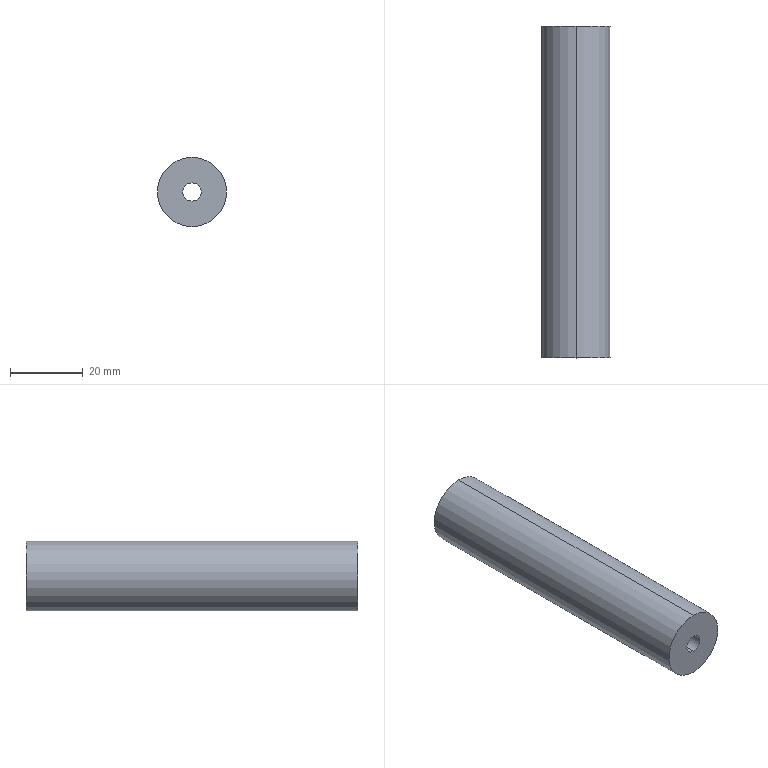Part | SolidWorks | features Extrusion 1, HoleWzd 1, ICE 1 | 1 solid | 9 faces | box 19 x 91 x 19 mm | volume 18359 mm3 | cylinder 6 | plane 3 | commonest cylinder face diameters 5 x2 11 x2 19 x2
STEP:
#1=CARTESIAN_POINT('',(0.,16.,-2.5));
#2=VERTEX_POINT('',#1);
#3=CARTESIAN_POINT('',(0.,16.,2.5));
#4=VERTEX_POINT('',#3);
#5=CARTESIAN_POINT('',(0.,16.,0.));
#6=DIRECTION('',(0.,1.,0.));
#7=DIRECTION('',(0.,0.,1.));
#8=AXIS2_PLACEMENT_3D('',#5,#6,#7);
#9=CIRCLE('',#8,2.5);
#10=EDGE_CURVE('',#2,#4,#9,.T.);
#11=ORIENTED_EDGE('',*,*,#10,.T.);
#12=CARTESIAN_POINT('',(0.,0.,2.5));
#13=VERTEX_POINT('',#12);
#14=CARTESIAN_POINT('',(0.,0.,2.5));
#15=DIRECTION('',(0.,-1.,0.));
#16=VECTOR('',#15,1000.);
#17=LINE('',#14,#16);
#18=EDGE_CURVE('',#4,#13,#17,.T.);
#19=ORIENTED_EDGE('',*,*,#18,.T.);
#20=CARTESIAN_POINT('',(0.,0.,-2.5));
#21=VERTEX_POINT('',#20);
#22=CARTESIAN_POINT('',(0.,0.,0.));
#23=DIRECTION('',(0.,-1.,0.));
#24=DIRECTION('',(0.,0.,-1.));
#25=AXIS2_PLACEMENT_3D('',#22,#23,#24);
#26=CIRCLE('',#25,2.5);
#27=EDGE_CURVE('',#13,#21,#26,.T.);
#28=ORIENTED_EDGE('',*,*,#27,.T.);
#29=CARTESIAN_POINT('',(0.,0.,-2.5));
#30=DIRECTION('',(0.,-1.,0.));
#31=VECTOR('',#30,1000.);
#32=LINE('',#29,#31);
#33=EDGE_CURVE('',#2,#21,#32,.T.);
#34=ORIENTED_EDGE('',*,*,#33,.F.);
#35=EDGE_LOOP('',(#11,#19,#28,#34));
#36=FACE_OUTER_BOUND('',#35,.T.);
#37=CARTESIAN_POINT('',(0.,0.,0.));
#38=DIRECTION('',(0.,-1.,0.));
#39=DIRECTION('',(0.,0.,-1.));
#40=AXIS2_PLACEMENT_3D('',#37,#38,#39);
#41=CYLINDRICAL_SURFACE('',#40,2.5);
#42=ADVANCED_FACE('',(#36),#41,.F.);
#43=CARTESIAN_POINT('',(0.,16.,-5.5));
#44=VERTEX_POINT('',#43);
#45=CARTESIAN_POINT('',(0.,16.,5.5));
#46=VERTEX_POINT('',#45);
#47=CARTESIAN_POINT('',(0.,16.,0.));
#48=DIRECTION('',(0.,1.,0.));
#49=DIRECTION('',(0.,0.,1.));
#50=AXIS2_PLACEMENT_3D('',#47,#48,#49);
#51=CIRCLE('',#50,5.5);
#52=EDGE_CURVE('',#44,#46,#51,.T.);
#53=ORIENTED_EDGE('',*,*,#52,.F.);
#54=CARTESIAN_POINT('',(0.,91.,-5.5));
#55=VERTEX_POINT('',#54);
#56=CARTESIAN_POINT('',(0.,16.,-5.5));
#57=DIRECTION('',(0.,1.,0.));
#58=VECTOR('',#57,1000.);
#59=LINE('',#56,#58);
#60=EDGE_CURVE('',#44,#55,#59,.T.);
#61=ORIENTED_EDGE('',*,*,#60,.T.);
#62=CARTESIAN_POINT('',(0.,91.,5.5));
#63=VERTEX_POINT('',#62);
#64=CARTESIAN_POINT('',(0.,91.,0.));
#65=DIRECTION('',(0.,1.,0.));
#66=DIRECTION('',(0.,0.,1.));
#67=AXIS2_PLACEMENT_3D('',#64,#65,#66);
#68=CIRCLE('',#67,5.5);
#69=EDGE_CURVE('',#55,#63,#68,.T.);
#70=ORIENTED_EDGE('',*,*,#69,.T.);
#71=CARTESIAN_POINT('',(0.,16.,5.5));
#72=DIRECTION('',(0.,1.,0.));
#73=VECTOR('',#72,1000.);
#74=LINE('',#71,#73);
#75=EDGE_CURVE('',#46,#63,#74,.T.);
#76=ORIENTED_EDGE('',*,*,#75,.F.);
#77=EDGE_LOOP('',(#53,#61,#70,#76));
#78=FACE_OUTER_BOUND('',#77,.T.);
#79=CARTESIAN_POINT('',(0.,16.,0.));
#80=DIRECTION('',(0.,1.,0.));
#81=DIRECTION('',(0.,0.,1.));
#82=AXIS2_PLACEMENT_3D('',#79,#80,#81);
#83=CYLINDRICAL_SURFACE('',#82,5.5);
#84=ADVANCED_FACE('',(#78),#83,.F.);
#85=CARTESIAN_POINT('',(0.,91.,9.5));
#86=VERTEX_POINT('',#85);
#87=CARTESIAN_POINT('',(0.,91.,-9.5));
#88=VERTEX_POINT('',#87);
#89=CARTESIAN_POINT('',(0.,91.,0.));
#90=DIRECTION('',(0.,1.,0.));
#91=DIRECTION('',(0.,0.,1.));
#92=AXIS2_PLACEMENT_3D('',#89,#90,#91);
#93=CIRCLE('',#92,9.5);
#94=EDGE_CURVE('',#86,#88,#93,.T.);
#95=ORIENTED_EDGE('',*,*,#94,.F.);
#96=CARTESIAN_POINT('',(0.,0.,9.5));
#97=VERTEX_POINT('',#96);
#98=CARTESIAN_POINT('',(0.,91.,9.5));
#99=DIRECTION('',(0.,-1.,0.));
#100=VECTOR('',#99,1000.);
#101=LINE('',#98,#100);
#102=EDGE_CURVE('',#86,#97,#101,.T.);
#103=ORIENTED_EDGE('',*,*,#102,.T.);
#104=CARTESIAN_POINT('',(0.,0.,-9.5));
#105=VERTEX_POINT('',#104);
#106=CARTESIAN_POINT('',(0.,0.,0.));
#107=DIRECTION('',(0.,1.,0.));
#108=DIRECTION('',(0.,0.,1.));
#109=AXIS2_PLACEMENT_3D('',#106,#107,#108);
#110=CIRCLE('',#109,9.5);
#111=EDGE_CURVE('',#97,#105,#110,.T.);
#112=ORIENTED_EDGE('',*,*,#111,.T.);
#113=CARTESIAN_POINT('',(0.,91.,-9.5));
#114=DIRECTION('',(0.,-1.,0.));
#115=VECTOR('',#114,1000.);
#116=LINE('',#113,#115);
#117=EDGE_CURVE('',#88,#105,#116,.T.);
#118=ORIENTED_EDGE('',*,*,#117,.F.);
#119=EDGE_LOOP('',(#95,#103,#112,#118));
#120=FACE_OUTER_BOUND('',#119,.T.);
#121=CARTESIAN_POINT('',(0.,91.,0.));
#122=DIRECTION('',(0.,-1.,0.));
#123=DIRECTION('',(0.,0.,-1.));
#124=AXIS2_PLACEMENT_3D('',#121,#122,#123);
#125=CYLINDRICAL_SURFACE('',#124,9.5);
#126=ADVANCED_FACE('',(#120),#125,.T.);
#127=ORIENTED_EDGE('',*,*,#102,.F.);
#128=CARTESIAN_POINT('',(0.,91.,0.));
#129=DIRECTION('',(0.,1.,0.));
#130=DIRECTION('',(0.,0.,1.));
#131=AXIS2_PLACEMENT_3D('',#128,#129,#130);
#132=CIRCLE('',#131,9.5);
#133=EDGE_CURVE('',#88,#86,#132,.T.);
#134=ORIENTED_EDGE('',*,*,#133,.F.);
#135=ORIENTED_EDGE('',*,*,#117,.T.);
#136=CARTESIAN_POINT('',(0.,0.,0.));
#137=DIRECTION('',(0.,1.,0.));
#138=DIRECTION('',(0.,0.,1.));
#139=AXIS2_PLACEMENT_3D('',#136,#137,#138);
#140=CIRCLE('',#139,9.5);
#141=EDGE_CURVE('',#105,#97,#140,.T.);
#142=ORIENTED_EDGE('',*,*,#141,.T.);
#143=EDGE_LOOP('',(#127,#134,#135,#142));
#144=FACE_OUTER_BOUND('',#143,.T.);
#145=CARTESIAN_POINT('',(0.,91.,0.));
#146=DIRECTION('',(0.,-1.,0.));
#147=DIRECTION('',(0.,0.,-1.));
#148=AXIS2_PLACEMENT_3D('',#145,#146,#147);
#149=CYLINDRICAL_SURFACE('',#148,9.5);
#150=ADVANCED_FACE('',(#144),#149,.T.);
#151=CARTESIAN_POINT('',(0.,91.,0.));
#152=DIRECTION('',(0.,1.,0.));
#153=DIRECTION('',(0.,0.,1.));
#154=AXIS2_PLACEMENT_3D('',#151,#152,#153);
#155=CIRCLE('',#154,5.5);
#156=EDGE_CURVE('',#63,#55,#155,.T.);
#157=ORIENTED_EDGE('',*,*,#156,.F.);
#158=ORIENTED_EDGE('',*,*,#69,.F.);
#159=EDGE_LOOP('',(#157,#158));
#160=FACE_BOUND('',#159,.T.);
#161=ORIENTED_EDGE('',*,*,#133,.T.);
#162=ORIENTED_EDGE('',*,*,#94,.T.);
#163=EDGE_LOOP('',(#161,#162));
#164=FACE_OUTER_BOUND('',#163,.T.);
#165=CARTESIAN_POINT('',(0.,91.,0.));
#166=DIRECTION('',(0.,1.,0.));
#167=DIRECTION('',(0.,0.,1.));
#168=AXIS2_PLACEMENT_3D('',#165,#166,#167);
#169=PLANE('',#168);
#170=ADVANCED_FACE('',(#160,#164),#169,.T.);
#171=CARTESIAN_POINT('',(0.,0.,0.));
#172=DIRECTION('',(0.,-1.,0.));
#173=DIRECTION('',(0.,0.,-1.));
#174=AXIS2_PLACEMENT_3D('',#171,#172,#173);
#175=CIRCLE('',#174,2.5);
#176=EDGE_CURVE('',#21,#13,#175,.T.);
#177=ORIENTED_EDGE('',*,*,#176,.F.);
#178=ORIENTED_EDGE('',*,*,#27,.F.);
#179=EDGE_LOOP('',(#177,#178));
#180=FACE_BOUND('',#179,.T.);
#181=ORIENTED_EDGE('',*,*,#141,.F.);
#182=ORIENTED_EDGE('',*,*,#111,.F.);
#183=EDGE_LOOP('',(#181,#182));
#184=FACE_OUTER_BOUND('',#183,.T.);
#185=CARTESIAN_POINT('',(0.,0.,0.));
#186=DIRECTION('',(0.,1.,0.));
#187=DIRECTION('',(0.,0.,1.));
#188=AXIS2_PLACEMENT_3D('',#185,#186,#187);
#189=PLANE('',#188);
#190=ADVANCED_FACE('',(#180,#184),#189,.F.);
#191=ORIENTED_EDGE('',*,*,#60,.F.);
#192=CARTESIAN_POINT('',(0.,16.,0.));
#193=DIRECTION('',(0.,1.,0.));
#194=DIRECTION('',(0.,0.,1.));
#195=AXIS2_PLACEMENT_3D('',#192,#193,#194);
#196=CIRCLE('',#195,5.5);
#197=EDGE_CURVE('',#46,#44,#196,.T.);
#198=ORIENTED_EDGE('',*,*,#197,.F.);
#199=ORIENTED_EDGE('',*,*,#75,.T.);
#200=ORIENTED_EDGE('',*,*,#156,.T.);
#201=EDGE_LOOP('',(#191,#198,#199,#200));
#202=FACE_OUTER_BOUND('',#201,.T.);
#203=CARTESIAN_POINT('',(0.,16.,0.));
#204=DIRECTION('',(0.,1.,0.));
#205=DIRECTION('',(0.,0.,1.));
#206=AXIS2_PLACEMENT_3D('',#203,#204,#205);
#207=CYLINDRICAL_SURFACE('',#206,5.5);
#208=ADVANCED_FACE('',(#202),#207,.F.);
#209=ORIENTED_EDGE('',*,*,#10,.F.);
#210=CARTESIAN_POINT('',(0.,16.,0.));
#211=DIRECTION('',(0.,1.,0.));
#212=DIRECTION('',(0.,0.,1.));
#213=AXIS2_PLACEMENT_3D('',#210,#211,#212);
#214=CIRCLE('',#213,2.5);
#215=EDGE_CURVE('',#4,#2,#214,.T.);
#216=ORIENTED_EDGE('',*,*,#215,.F.);
#217=EDGE_LOOP('',(#209,#216));
#218=FACE_BOUND('',#217,.T.);
#219=ORIENTED_EDGE('',*,*,#197,.T.);
#220=ORIENTED_EDGE('',*,*,#52,.T.);
#221=EDGE_LOOP('',(#219,#220));
#222=FACE_OUTER_BOUND('',#221,.T.);
#223=CARTESIAN_POINT('',(0.,16.,0.));
#224=DIRECTION('',(0.,1.,0.));
#225=DIRECTION('',(0.,0.,1.));
#226=AXIS2_PLACEMENT_3D('',#223,#224,#225);
#227=PLANE('',#226);
#228=ADVANCED_FACE('',(#218,#222),#227,.T.);
#229=ORIENTED_EDGE('',*,*,#18,.F.);
#230=ORIENTED_EDGE('',*,*,#215,.T.);
#231=ORIENTED_EDGE('',*,*,#33,.T.);
#232=ORIENTED_EDGE('',*,*,#176,.T.);
#233=EDGE_LOOP('',(#229,#230,#231,#232));
#234=FACE_OUTER_BOUND('',#233,.T.);
#235=CARTESIAN_POINT('',(0.,0.,0.));
#236=DIRECTION('',(0.,-1.,0.));
#237=DIRECTION('',(0.,0.,-1.));
#238=AXIS2_PLACEMENT_3D('',#235,#236,#237);
#239=CYLINDRICAL_SURFACE('',#238,2.5);
#240=ADVANCED_FACE('',(#234),#239,.F.);
#241=CLOSED_SHELL('',(#42,#84,#126,#150,#170,#190,#208,#228,#240));
#242=MANIFOLD_SOLID_BREP('',#241);
#243=CARTESIAN_POINT('',(0.,0.,0.));
#244=DIRECTION('',(0.,0.,1.));
#245=DIRECTION('',(1.,0.,0.));
#246=AXIS2_PLACEMENT_3D('',#243,#244,#245);
#247=(LENGTH_UNIT()NAMED_UNIT(*)SI_UNIT(.MILLI.,.METRE.));
#248=UNCERTAINTY_MEASURE_WITH_UNIT(LENGTH_MEASURE(0.00001),#247,'','');
#249=(NAMED_UNIT(*)PLANE_ANGLE_UNIT()SI_UNIT($,.RADIAN.));
#250=(NAMED_UNIT(*)SI_UNIT($,.STERADIAN.)SOLID_ANGLE_UNIT());
#251=(GEOMETRIC_REPRESENTATION_CONTEXT(3)GLOBAL_UNCERTAINTY_ASSIGNED_CONTEXT((#248))GLOBAL_UNIT_ASSIGNED_CONTEXT((#247,#249,#250))REPRESENTATION_CONTEXT('',''));
#252=ADVANCED_BREP_SHAPE_REPRESENTATION('',(#242,#246),#251);